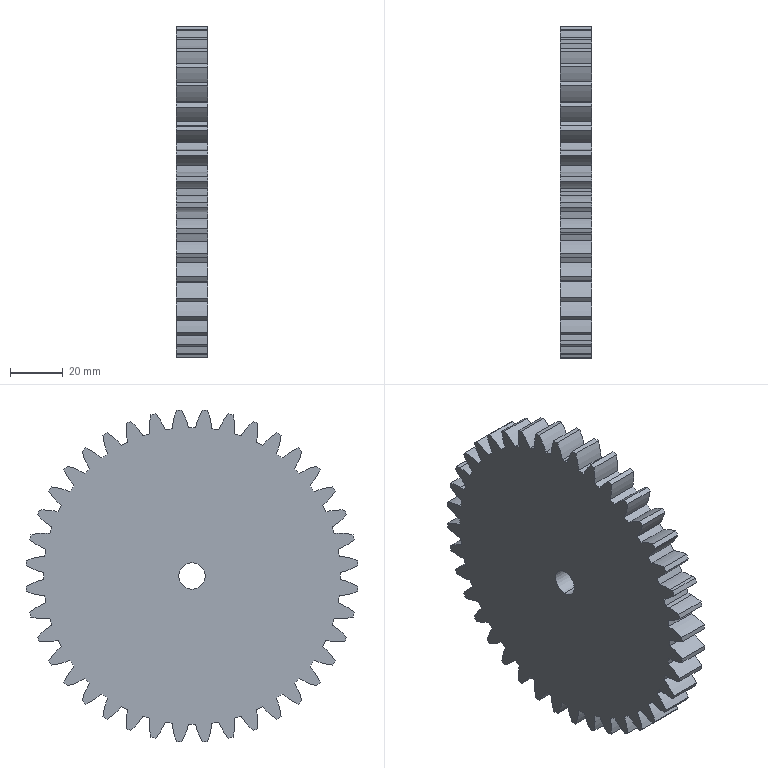Part | SolidWorks | features Boss 3, Cut 3, CirPattern 2, Fillet 2, Revolution 1 | 1 solid | 169 faces | box 12 x 125.745 x 125.745 mm | volume 132575 mm3 | cylinder 167 | plane 2 | commonest cylinder face diameters 48 x84 112.498 x41 126 x40 10 x2